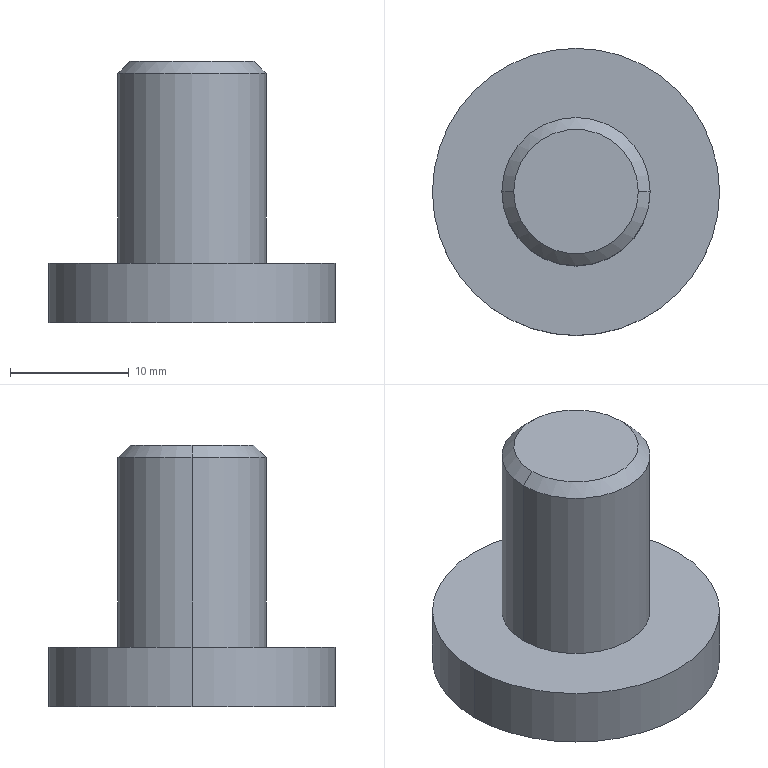Part | SolidWorks | features Chamfer 1, Extrusion 1, ICE 1 | 1 solid | 9 faces | box 24.181 x 24.181 x 22 mm | volume 4364 mm3 | cylinder 4 | plane 3 | cone 2 | commonest cylinder face diameters 12.5 x2 24.181 x2
STEP:
#1=CARTESIAN_POINT('',(5.25,0.,22.));
#2=VERTEX_POINT('',#1);
#3=CARTESIAN_POINT('',(-5.25,0.,22.));
#4=VERTEX_POINT('',#3);
#5=CARTESIAN_POINT('',(0.,0.,22.));
#6=DIRECTION('',(0.,0.,1.));
#7=DIRECTION('',(1.,0.,0.));
#8=AXIS2_PLACEMENT_3D('',#5,#6,#7);
#9=CIRCLE('',#8,5.25);
#10=EDGE_CURVE('',#2,#4,#9,.T.);
#11=ORIENTED_EDGE('',*,*,#10,.F.);
#12=CARTESIAN_POINT('',(6.25,0.,21.));
#13=VERTEX_POINT('',#12);
#14=CARTESIAN_POINT('',(5.25,0.,22.));
#15=DIRECTION('',(0.7071,0.,-0.7071));
#16=VECTOR('',#15,1000.);
#17=LINE('',#14,#16);
#18=EDGE_CURVE('',#2,#13,#17,.T.);
#19=ORIENTED_EDGE('',*,*,#18,.T.);
#20=CARTESIAN_POINT('',(-6.25,0.,21.));
#21=VERTEX_POINT('',#20);
#22=CARTESIAN_POINT('',(0.,0.,21.));
#23=DIRECTION('',(0.,0.,-1.));
#24=DIRECTION('',(1.,0.,0.));
#25=AXIS2_PLACEMENT_3D('',#22,#23,#24);
#26=CIRCLE('',#25,6.25);
#27=EDGE_CURVE('',#21,#13,#26,.T.);
#28=ORIENTED_EDGE('',*,*,#27,.F.);
#29=CARTESIAN_POINT('',(-5.25,0.,22.));
#30=DIRECTION('',(-0.7071,0.,-0.7071));
#31=VECTOR('',#30,1000.);
#32=LINE('',#29,#31);
#33=EDGE_CURVE('',#4,#21,#32,.T.);
#34=ORIENTED_EDGE('',*,*,#33,.F.);
#35=EDGE_LOOP('',(#11,#19,#28,#34));
#36=FACE_OUTER_BOUND('',#35,.T.);
#37=CARTESIAN_POINT('',(0.,0.,22.));
#38=DIRECTION('',(0.,0.,-1.));
#39=DIRECTION('',(-1.,0.,0.));
#40=AXIS2_PLACEMENT_3D('',#37,#38,#39);
#41=CONICAL_SURFACE('',#40,5.25,0.7854);
#42=ADVANCED_FACE('',(#36),#41,.T.);
#43=ORIENTED_EDGE('',*,*,#27,.T.);
#44=CARTESIAN_POINT('',(6.25,0.,5.));
#45=VERTEX_POINT('',#44);
#46=CARTESIAN_POINT('',(6.25,0.,22.));
#47=DIRECTION('',(0.,0.,-1.));
#48=VECTOR('',#47,1000.);
#49=LINE('',#46,#48);
#50=EDGE_CURVE('',#13,#45,#49,.T.);
#51=ORIENTED_EDGE('',*,*,#50,.T.);
#52=CARTESIAN_POINT('',(-6.25,0.,5.));
#53=VERTEX_POINT('',#52);
#54=CARTESIAN_POINT('',(0.,0.,5.));
#55=DIRECTION('',(0.,0.,1.));
#56=DIRECTION('',(1.,0.,0.));
#57=AXIS2_PLACEMENT_3D('',#54,#55,#56);
#58=CIRCLE('',#57,6.25);
#59=EDGE_CURVE('',#45,#53,#58,.T.);
#60=ORIENTED_EDGE('',*,*,#59,.T.);
#61=CARTESIAN_POINT('',(-6.25,0.,22.));
#62=DIRECTION('',(0.,0.,-1.));
#63=VECTOR('',#62,1000.);
#64=LINE('',#61,#63);
#65=EDGE_CURVE('',#21,#53,#64,.T.);
#66=ORIENTED_EDGE('',*,*,#65,.F.);
#67=EDGE_LOOP('',(#43,#51,#60,#66));
#68=FACE_OUTER_BOUND('',#67,.T.);
#69=CARTESIAN_POINT('',(0.,0.,22.));
#70=DIRECTION('',(0.,0.,-1.));
#71=DIRECTION('',(-1.,0.,0.));
#72=AXIS2_PLACEMENT_3D('',#69,#70,#71);
#73=CYLINDRICAL_SURFACE('',#72,6.25);
#74=ADVANCED_FACE('',(#68),#73,.T.);
#75=CARTESIAN_POINT('',(12.091,0.,5.));
#76=VERTEX_POINT('',#75);
#77=CARTESIAN_POINT('',(-12.091,0.,5.));
#78=VERTEX_POINT('',#77);
#79=CARTESIAN_POINT('',(0.,0.,5.));
#80=DIRECTION('',(0.,0.,1.));
#81=DIRECTION('',(1.,0.,0.));
#82=AXIS2_PLACEMENT_3D('',#79,#80,#81);
#83=CIRCLE('',#82,12.091);
#84=EDGE_CURVE('',#76,#78,#83,.T.);
#85=ORIENTED_EDGE('',*,*,#84,.F.);
#86=CARTESIAN_POINT('',(12.091,0.,0.));
#87=VERTEX_POINT('',#86);
#88=CARTESIAN_POINT('',(12.091,0.,5.));
#89=DIRECTION('',(0.,0.,-1.));
#90=VECTOR('',#89,1000.);
#91=LINE('',#88,#90);
#92=EDGE_CURVE('',#76,#87,#91,.T.);
#93=ORIENTED_EDGE('',*,*,#92,.T.);
#94=CARTESIAN_POINT('',(-12.091,0.,0.));
#95=VERTEX_POINT('',#94);
#96=CARTESIAN_POINT('',(0.,0.,0.));
#97=DIRECTION('',(0.,0.,1.));
#98=DIRECTION('',(1.,0.,0.));
#99=AXIS2_PLACEMENT_3D('',#96,#97,#98);
#100=CIRCLE('',#99,12.091);
#101=EDGE_CURVE('',#87,#95,#100,.T.);
#102=ORIENTED_EDGE('',*,*,#101,.T.);
#103=CARTESIAN_POINT('',(-12.091,0.,5.));
#104=DIRECTION('',(0.,0.,-1.));
#105=VECTOR('',#104,1000.);
#106=LINE('',#103,#105);
#107=EDGE_CURVE('',#78,#95,#106,.T.);
#108=ORIENTED_EDGE('',*,*,#107,.F.);
#109=EDGE_LOOP('',(#85,#93,#102,#108));
#110=FACE_OUTER_BOUND('',#109,.T.);
#111=CARTESIAN_POINT('',(0.,0.,5.));
#112=DIRECTION('',(0.,0.,-1.));
#113=DIRECTION('',(-1.,0.,0.));
#114=AXIS2_PLACEMENT_3D('',#111,#112,#113);
#115=CYLINDRICAL_SURFACE('',#114,12.091);
#116=ADVANCED_FACE('',(#110),#115,.T.);
#117=ORIENTED_EDGE('',*,*,#92,.F.);
#118=CARTESIAN_POINT('',(0.,0.,5.));
#119=DIRECTION('',(0.,0.,1.));
#120=DIRECTION('',(1.,0.,0.));
#121=AXIS2_PLACEMENT_3D('',#118,#119,#120);
#122=CIRCLE('',#121,12.091);
#123=EDGE_CURVE('',#78,#76,#122,.T.);
#124=ORIENTED_EDGE('',*,*,#123,.F.);
#125=ORIENTED_EDGE('',*,*,#107,.T.);
#126=CARTESIAN_POINT('',(0.,0.,0.));
#127=DIRECTION('',(0.,0.,1.));
#128=DIRECTION('',(1.,0.,0.));
#129=AXIS2_PLACEMENT_3D('',#126,#127,#128);
#130=CIRCLE('',#129,12.091);
#131=EDGE_CURVE('',#95,#87,#130,.T.);
#132=ORIENTED_EDGE('',*,*,#131,.T.);
#133=EDGE_LOOP('',(#117,#124,#125,#132));
#134=FACE_OUTER_BOUND('',#133,.T.);
#135=CARTESIAN_POINT('',(0.,0.,5.));
#136=DIRECTION('',(0.,0.,-1.));
#137=DIRECTION('',(-1.,0.,0.));
#138=AXIS2_PLACEMENT_3D('',#135,#136,#137);
#139=CYLINDRICAL_SURFACE('',#138,12.091);
#140=ADVANCED_FACE('',(#134),#139,.T.);
#141=CARTESIAN_POINT('',(0.,0.,5.));
#142=DIRECTION('',(0.,0.,1.));
#143=DIRECTION('',(1.,0.,0.));
#144=AXIS2_PLACEMENT_3D('',#141,#142,#143);
#145=CIRCLE('',#144,6.25);
#146=EDGE_CURVE('',#53,#45,#145,.T.);
#147=ORIENTED_EDGE('',*,*,#146,.F.);
#148=ORIENTED_EDGE('',*,*,#59,.F.);
#149=EDGE_LOOP('',(#147,#148));
#150=FACE_BOUND('',#149,.T.);
#151=ORIENTED_EDGE('',*,*,#123,.T.);
#152=ORIENTED_EDGE('',*,*,#84,.T.);
#153=EDGE_LOOP('',(#151,#152));
#154=FACE_OUTER_BOUND('',#153,.T.);
#155=CARTESIAN_POINT('',(0.,0.,5.));
#156=DIRECTION('',(0.,0.,1.));
#157=DIRECTION('',(1.,0.,0.));
#158=AXIS2_PLACEMENT_3D('',#155,#156,#157);
#159=PLANE('',#158);
#160=ADVANCED_FACE('',(#150,#154),#159,.T.);
#161=ORIENTED_EDGE('',*,*,#131,.F.);
#162=ORIENTED_EDGE('',*,*,#101,.F.);
#163=EDGE_LOOP('',(#161,#162));
#164=FACE_OUTER_BOUND('',#163,.T.);
#165=CARTESIAN_POINT('',(0.,0.,0.));
#166=DIRECTION('',(0.,0.,1.));
#167=DIRECTION('',(1.,0.,0.));
#168=AXIS2_PLACEMENT_3D('',#165,#166,#167);
#169=PLANE('',#168);
#170=ADVANCED_FACE('',(#164),#169,.F.);
#171=ORIENTED_EDGE('',*,*,#50,.F.);
#172=CARTESIAN_POINT('',(0.,0.,21.));
#173=DIRECTION('',(0.,0.,-1.));
#174=DIRECTION('',(1.,0.,0.));
#175=AXIS2_PLACEMENT_3D('',#172,#173,#174);
#176=CIRCLE('',#175,6.25);
#177=EDGE_CURVE('',#13,#21,#176,.T.);
#178=ORIENTED_EDGE('',*,*,#177,.T.);
#179=ORIENTED_EDGE('',*,*,#65,.T.);
#180=ORIENTED_EDGE('',*,*,#146,.T.);
#181=EDGE_LOOP('',(#171,#178,#179,#180));
#182=FACE_OUTER_BOUND('',#181,.T.);
#183=CARTESIAN_POINT('',(0.,0.,22.));
#184=DIRECTION('',(0.,0.,-1.));
#185=DIRECTION('',(-1.,0.,0.));
#186=AXIS2_PLACEMENT_3D('',#183,#184,#185);
#187=CYLINDRICAL_SURFACE('',#186,6.25);
#188=ADVANCED_FACE('',(#182),#187,.T.);
#189=CARTESIAN_POINT('',(0.,0.,22.));
#190=DIRECTION('',(0.,0.,1.));
#191=DIRECTION('',(1.,0.,0.));
#192=AXIS2_PLACEMENT_3D('',#189,#190,#191);
#193=CIRCLE('',#192,5.25);
#194=EDGE_CURVE('',#4,#2,#193,.T.);
#195=ORIENTED_EDGE('',*,*,#194,.T.);
#196=ORIENTED_EDGE('',*,*,#10,.T.);
#197=EDGE_LOOP('',(#195,#196));
#198=FACE_OUTER_BOUND('',#197,.T.);
#199=CARTESIAN_POINT('',(0.,0.,22.));
#200=DIRECTION('',(0.,0.,1.));
#201=DIRECTION('',(1.,0.,0.));
#202=AXIS2_PLACEMENT_3D('',#199,#200,#201);
#203=PLANE('',#202);
#204=ADVANCED_FACE('',(#198),#203,.T.);
#205=ORIENTED_EDGE('',*,*,#18,.F.);
#206=ORIENTED_EDGE('',*,*,#194,.F.);
#207=ORIENTED_EDGE('',*,*,#33,.T.);
#208=ORIENTED_EDGE('',*,*,#177,.F.);
#209=EDGE_LOOP('',(#205,#206,#207,#208));
#210=FACE_OUTER_BOUND('',#209,.T.);
#211=CARTESIAN_POINT('',(0.,0.,22.));
#212=DIRECTION('',(0.,0.,-1.));
#213=DIRECTION('',(-1.,0.,0.));
#214=AXIS2_PLACEMENT_3D('',#211,#212,#213);
#215=CONICAL_SURFACE('',#214,5.25,0.7854);
#216=ADVANCED_FACE('',(#210),#215,.T.);
#217=CLOSED_SHELL('',(#42,#74,#116,#140,#160,#170,#188,#204,#216));
#218=MANIFOLD_SOLID_BREP('',#217);
#219=CARTESIAN_POINT('',(0.,0.,0.));
#220=DIRECTION('',(0.,0.,1.));
#221=DIRECTION('',(1.,0.,0.));
#222=AXIS2_PLACEMENT_3D('',#219,#220,#221);
#223=(LENGTH_UNIT()NAMED_UNIT(*)SI_UNIT(.MILLI.,.METRE.));
#224=UNCERTAINTY_MEASURE_WITH_UNIT(LENGTH_MEASURE(0.00001),#223,'','');
#225=(NAMED_UNIT(*)PLANE_ANGLE_UNIT()SI_UNIT($,.RADIAN.));
#226=(NAMED_UNIT(*)SI_UNIT($,.STERADIAN.)SOLID_ANGLE_UNIT());
#227=(GEOMETRIC_REPRESENTATION_CONTEXT(3)GLOBAL_UNCERTAINTY_ASSIGNED_CONTEXT((#224))GLOBAL_UNIT_ASSIGNED_CONTEXT((#223,#225,#226))REPRESENTATION_CONTEXT('',''));
#228=ADVANCED_BREP_SHAPE_REPRESENTATION('',(#218,#222),#227);